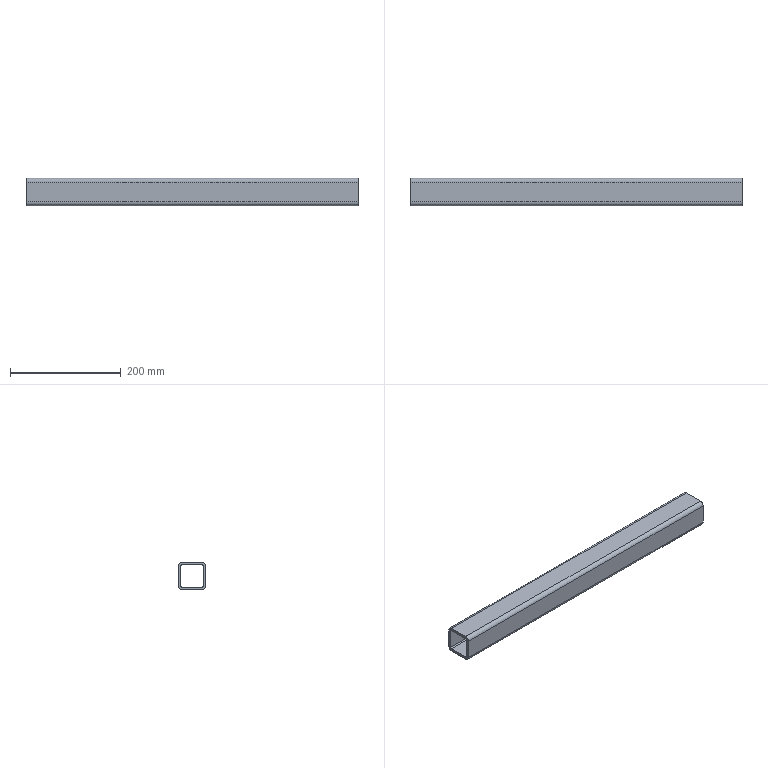Part | NX | 1 solid | 18 faces | box 600 x 50 x 50 mm | volume 516823 mm3 | plane 10 | cylinder 8 | commonest cylinder face diameters 4 x4 14 x4
STEP:
#1=CARTESIAN_POINT('',(950.,838.,20.));
#2=VERTEX_POINT('',#1);
#3=CARTESIAN_POINT('',(350.,838.,20.));
#4=VERTEX_POINT('',#3);
#5=CARTESIAN_POINT('',(975.,838.,20.));
#6=DIRECTION('',(-1.,0.,0.));
#7=VECTOR('',#6,1000.);
#8=LINE('',#5,#7);
#9=EDGE_CURVE('',#2,#4,#8,.T.);
#10=ORIENTED_EDGE('',*,*,#9,.T.);
#11=CARTESIAN_POINT('',(350.,874.,20.));
#12=VERTEX_POINT('',#11);
#13=CARTESIAN_POINT('',(350.,838.,20.));
#14=DIRECTION('',(0.,1.,0.));
#15=VECTOR('',#14,1000.);
#16=LINE('',#13,#15);
#17=EDGE_CURVE('',#4,#12,#16,.T.);
#18=ORIENTED_EDGE('',*,*,#17,.T.);
#19=CARTESIAN_POINT('',(950.,874.,20.));
#20=VERTEX_POINT('',#19);
#21=CARTESIAN_POINT('',(975.,874.,20.));
#22=DIRECTION('',(-1.,0.,0.));
#23=VECTOR('',#22,1000.);
#24=LINE('',#21,#23);
#25=EDGE_CURVE('',#20,#12,#24,.T.);
#26=ORIENTED_EDGE('',*,*,#25,.F.);
#27=CARTESIAN_POINT('',(950.,838.,20.));
#28=DIRECTION('',(0.,-1.,0.));
#29=VECTOR('',#28,1000.);
#30=LINE('',#27,#29);
#31=EDGE_CURVE('',#20,#2,#30,.T.);
#32=ORIENTED_EDGE('',*,*,#31,.T.);
#33=EDGE_LOOP('',(#10,#18,#26,#32));
#34=FACE_BOUND('',#33,.T.);
#35=CARTESIAN_POINT('',(975.,838.,20.));
#36=DIRECTION('',(0.,0.,-1.));
#37=DIRECTION('',(0.,1.,0.));
#38=AXIS2_PLACEMENT_3D('',#35,#36,#37);
#39=PLANE('',#38);
#40=ADVANCED_FACE('',(#34),#39,.T.);
#41=CARTESIAN_POINT('',(950.,836.,18.));
#42=VERTEX_POINT('',#41);
#43=CARTESIAN_POINT('',(350.,836.,18.));
#44=VERTEX_POINT('',#43);
#45=CARTESIAN_POINT('',(975.,836.,18.));
#46=DIRECTION('',(-1.,0.,0.));
#47=VECTOR('',#46,1000.);
#48=LINE('',#45,#47);
#49=EDGE_CURVE('',#42,#44,#48,.T.);
#50=ORIENTED_EDGE('',*,*,#49,.T.);
#51=CARTESIAN_POINT('',(350.,838.,18.));
#52=DIRECTION('',(-1.,0.,0.));
#53=DIRECTION('',(0.,-1.,0.));
#54=AXIS2_PLACEMENT_3D('',#51,#52,#53);
#55=CIRCLE('',#54,2.);
#56=EDGE_CURVE('',#44,#4,#55,.T.);
#57=ORIENTED_EDGE('',*,*,#56,.T.);
#58=ORIENTED_EDGE('',*,*,#9,.F.);
#59=CARTESIAN_POINT('',(950.,838.,18.));
#60=DIRECTION('',(1.,0.,0.));
#61=DIRECTION('',(0.,1.,0.));
#62=AXIS2_PLACEMENT_3D('',#59,#60,#61);
#63=CIRCLE('',#62,2.);
#64=EDGE_CURVE('',#2,#42,#63,.T.);
#65=ORIENTED_EDGE('',*,*,#64,.T.);
#66=EDGE_LOOP('',(#50,#57,#58,#65));
#67=FACE_BOUND('',#66,.T.);
#68=CARTESIAN_POINT('',(975.,838.,18.));
#69=DIRECTION('',(-1.,0.,0.));
#70=DIRECTION('',(0.,0.,1.));
#71=AXIS2_PLACEMENT_3D('',#68,#69,#70);
#72=CYLINDRICAL_SURFACE('',#71,2.);
#73=ADVANCED_FACE('',(#67),#72,.F.);
#74=CARTESIAN_POINT('',(950.,836.,-18.));
#75=VERTEX_POINT('',#74);
#76=CARTESIAN_POINT('',(350.,836.,-18.));
#77=VERTEX_POINT('',#76);
#78=CARTESIAN_POINT('',(975.,836.,-18.));
#79=DIRECTION('',(-1.,0.,0.));
#80=VECTOR('',#79,1000.);
#81=LINE('',#78,#80);
#82=EDGE_CURVE('',#75,#77,#81,.T.);
#83=ORIENTED_EDGE('',*,*,#82,.T.);
#84=CARTESIAN_POINT('',(350.,836.,18.));
#85=DIRECTION('',(0.,0.,1.));
#86=VECTOR('',#85,1000.);
#87=LINE('',#84,#86);
#88=EDGE_CURVE('',#77,#44,#87,.T.);
#89=ORIENTED_EDGE('',*,*,#88,.T.);
#90=ORIENTED_EDGE('',*,*,#49,.F.);
#91=CARTESIAN_POINT('',(950.,836.,18.));
#92=DIRECTION('',(0.,0.,-1.));
#93=VECTOR('',#92,1000.);
#94=LINE('',#91,#93);
#95=EDGE_CURVE('',#42,#75,#94,.T.);
#96=ORIENTED_EDGE('',*,*,#95,.T.);
#97=EDGE_LOOP('',(#83,#89,#90,#96));
#98=FACE_BOUND('',#97,.T.);
#99=CARTESIAN_POINT('',(975.,836.,18.));
#100=DIRECTION('',(0.,1.,0.));
#101=DIRECTION('',(0.,0.,1.));
#102=AXIS2_PLACEMENT_3D('',#99,#100,#101);
#103=PLANE('',#102);
#104=ADVANCED_FACE('',(#98),#103,.T.);
#105=CARTESIAN_POINT('',(950.,838.,-20.));
#106=VERTEX_POINT('',#105);
#107=CARTESIAN_POINT('',(350.,838.,-20.));
#108=VERTEX_POINT('',#107);
#109=CARTESIAN_POINT('',(975.,838.,-20.));
#110=DIRECTION('',(-1.,0.,0.));
#111=VECTOR('',#110,1000.);
#112=LINE('',#109,#111);
#113=EDGE_CURVE('',#106,#108,#112,.T.);
#114=ORIENTED_EDGE('',*,*,#113,.T.);
#115=CARTESIAN_POINT('',(350.,838.,-18.));
#116=DIRECTION('',(-1.,0.,0.));
#117=DIRECTION('',(0.,-1.,0.));
#118=AXIS2_PLACEMENT_3D('',#115,#116,#117);
#119=CIRCLE('',#118,2.);
#120=EDGE_CURVE('',#108,#77,#119,.T.);
#121=ORIENTED_EDGE('',*,*,#120,.T.);
#122=ORIENTED_EDGE('',*,*,#82,.F.);
#123=CARTESIAN_POINT('',(950.,838.,-18.));
#124=DIRECTION('',(1.,0.,0.));
#125=DIRECTION('',(0.,1.,0.));
#126=AXIS2_PLACEMENT_3D('',#123,#124,#125);
#127=CIRCLE('',#126,2.);
#128=EDGE_CURVE('',#75,#106,#127,.T.);
#129=ORIENTED_EDGE('',*,*,#128,.T.);
#130=EDGE_LOOP('',(#114,#121,#122,#129));
#131=FACE_BOUND('',#130,.T.);
#132=CARTESIAN_POINT('',(975.,838.,-18.));
#133=DIRECTION('',(-1.,0.,0.));
#134=DIRECTION('',(0.,0.,1.));
#135=AXIS2_PLACEMENT_3D('',#132,#133,#134);
#136=CYLINDRICAL_SURFACE('',#135,2.);
#137=ADVANCED_FACE('',(#131),#136,.F.);
#138=CARTESIAN_POINT('',(950.,874.,-20.));
#139=VERTEX_POINT('',#138);
#140=CARTESIAN_POINT('',(350.,874.,-20.));
#141=VERTEX_POINT('',#140);
#142=CARTESIAN_POINT('',(975.,874.,-20.));
#143=DIRECTION('',(-1.,0.,0.));
#144=VECTOR('',#143,1000.);
#145=LINE('',#142,#144);
#146=EDGE_CURVE('',#139,#141,#145,.T.);
#147=ORIENTED_EDGE('',*,*,#146,.T.);
#148=CARTESIAN_POINT('',(350.,874.,-20.));
#149=DIRECTION('',(0.,-1.,0.));
#150=VECTOR('',#149,1000.);
#151=LINE('',#148,#150);
#152=EDGE_CURVE('',#141,#108,#151,.T.);
#153=ORIENTED_EDGE('',*,*,#152,.T.);
#154=ORIENTED_EDGE('',*,*,#113,.F.);
#155=CARTESIAN_POINT('',(950.,874.,-20.));
#156=DIRECTION('',(0.,1.,0.));
#157=VECTOR('',#156,1000.);
#158=LINE('',#155,#157);
#159=EDGE_CURVE('',#106,#139,#158,.T.);
#160=ORIENTED_EDGE('',*,*,#159,.T.);
#161=EDGE_LOOP('',(#147,#153,#154,#160));
#162=FACE_BOUND('',#161,.T.);
#163=CARTESIAN_POINT('',(975.,874.,-20.));
#164=DIRECTION('',(0.,0.,1.));
#165=DIRECTION('',(0.,-1.,0.));
#166=AXIS2_PLACEMENT_3D('',#163,#164,#165);
#167=PLANE('',#166);
#168=ADVANCED_FACE('',(#162),#167,.T.);
#169=CARTESIAN_POINT('',(950.,876.,-18.));
#170=VERTEX_POINT('',#169);
#171=CARTESIAN_POINT('',(350.,876.,-18.));
#172=VERTEX_POINT('',#171);
#173=CARTESIAN_POINT('',(975.,876.,-18.));
#174=DIRECTION('',(-1.,0.,0.));
#175=VECTOR('',#174,1000.);
#176=LINE('',#173,#175);
#177=EDGE_CURVE('',#170,#172,#176,.T.);
#178=ORIENTED_EDGE('',*,*,#177,.T.);
#179=CARTESIAN_POINT('',(350.,874.,-18.));
#180=DIRECTION('',(-1.,0.,0.));
#181=DIRECTION('',(0.,-1.,0.));
#182=AXIS2_PLACEMENT_3D('',#179,#180,#181);
#183=CIRCLE('',#182,2.);
#184=EDGE_CURVE('',#172,#141,#183,.T.);
#185=ORIENTED_EDGE('',*,*,#184,.T.);
#186=ORIENTED_EDGE('',*,*,#146,.F.);
#187=CARTESIAN_POINT('',(950.,874.,-18.));
#188=DIRECTION('',(1.,0.,0.));
#189=DIRECTION('',(0.,1.,0.));
#190=AXIS2_PLACEMENT_3D('',#187,#188,#189);
#191=CIRCLE('',#190,2.);
#192=EDGE_CURVE('',#139,#170,#191,.T.);
#193=ORIENTED_EDGE('',*,*,#192,.T.);
#194=EDGE_LOOP('',(#178,#185,#186,#193));
#195=FACE_BOUND('',#194,.T.);
#196=CARTESIAN_POINT('',(975.,874.,-18.));
#197=DIRECTION('',(-1.,0.,0.));
#198=DIRECTION('',(0.,0.,1.));
#199=AXIS2_PLACEMENT_3D('',#196,#197,#198);
#200=CYLINDRICAL_SURFACE('',#199,2.);
#201=ADVANCED_FACE('',(#195),#200,.F.);
#202=CARTESIAN_POINT('',(950.,876.,18.));
#203=VERTEX_POINT('',#202);
#204=CARTESIAN_POINT('',(350.,876.,18.));
#205=VERTEX_POINT('',#204);
#206=CARTESIAN_POINT('',(975.,876.,18.));
#207=DIRECTION('',(-1.,0.,0.));
#208=VECTOR('',#207,1000.);
#209=LINE('',#206,#208);
#210=EDGE_CURVE('',#203,#205,#209,.T.);
#211=ORIENTED_EDGE('',*,*,#210,.T.);
#212=CARTESIAN_POINT('',(350.,876.,-18.));
#213=DIRECTION('',(0.,0.,-1.));
#214=VECTOR('',#213,1000.);
#215=LINE('',#212,#214);
#216=EDGE_CURVE('',#205,#172,#215,.T.);
#217=ORIENTED_EDGE('',*,*,#216,.T.);
#218=ORIENTED_EDGE('',*,*,#177,.F.);
#219=CARTESIAN_POINT('',(950.,876.,-18.));
#220=DIRECTION('',(0.,0.,1.));
#221=VECTOR('',#220,1000.);
#222=LINE('',#219,#221);
#223=EDGE_CURVE('',#170,#203,#222,.T.);
#224=ORIENTED_EDGE('',*,*,#223,.T.);
#225=EDGE_LOOP('',(#211,#217,#218,#224));
#226=FACE_BOUND('',#225,.T.);
#227=CARTESIAN_POINT('',(975.,876.,-18.));
#228=DIRECTION('',(0.,-1.,0.));
#229=DIRECTION('',(0.,0.,-1.));
#230=AXIS2_PLACEMENT_3D('',#227,#228,#229);
#231=PLANE('',#230);
#232=ADVANCED_FACE('',(#226),#231,.T.);
#233=ORIENTED_EDGE('',*,*,#25,.T.);
#234=CARTESIAN_POINT('',(350.,874.,18.));
#235=DIRECTION('',(-1.,0.,0.));
#236=DIRECTION('',(0.,-1.,0.));
#237=AXIS2_PLACEMENT_3D('',#234,#235,#236);
#238=CIRCLE('',#237,2.);
#239=EDGE_CURVE('',#12,#205,#238,.T.);
#240=ORIENTED_EDGE('',*,*,#239,.T.);
#241=ORIENTED_EDGE('',*,*,#210,.F.);
#242=CARTESIAN_POINT('',(950.,874.,18.));
#243=DIRECTION('',(1.,0.,0.));
#244=DIRECTION('',(0.,1.,0.));
#245=AXIS2_PLACEMENT_3D('',#242,#243,#244);
#246=CIRCLE('',#245,2.);
#247=EDGE_CURVE('',#203,#20,#246,.T.);
#248=ORIENTED_EDGE('',*,*,#247,.T.);
#249=EDGE_LOOP('',(#233,#240,#241,#248));
#250=FACE_BOUND('',#249,.T.);
#251=CARTESIAN_POINT('',(975.,874.,18.));
#252=DIRECTION('',(-1.,0.,0.));
#253=DIRECTION('',(0.,0.,1.));
#254=AXIS2_PLACEMENT_3D('',#251,#252,#253);
#255=CYLINDRICAL_SURFACE('',#254,2.);
#256=ADVANCED_FACE('',(#250),#255,.F.);
#257=CARTESIAN_POINT('',(350.,874.,-25.));
#258=VERTEX_POINT('',#257);
#259=CARTESIAN_POINT('',(350.,838.,-25.));
#260=VERTEX_POINT('',#259);
#261=CARTESIAN_POINT('',(350.,874.,-25.));
#262=DIRECTION('',(0.,-1.,0.));
#263=VECTOR('',#262,1000.);
#264=LINE('',#261,#263);
#265=EDGE_CURVE('',#258,#260,#264,.T.);
#266=ORIENTED_EDGE('',*,*,#265,.F.);
#267=CARTESIAN_POINT('',(950.,874.,-25.));
#268=VERTEX_POINT('',#267);
#269=CARTESIAN_POINT('',(975.,874.,-25.));
#270=DIRECTION('',(-1.,0.,0.));
#271=VECTOR('',#270,1000.);
#272=LINE('',#269,#271);
#273=EDGE_CURVE('',#268,#258,#272,.T.);
#274=ORIENTED_EDGE('',*,*,#273,.F.);
#275=CARTESIAN_POINT('',(950.,838.,-25.));
#276=VERTEX_POINT('',#275);
#277=CARTESIAN_POINT('',(950.,874.,-25.));
#278=DIRECTION('',(0.,1.,0.));
#279=VECTOR('',#278,1000.);
#280=LINE('',#277,#279);
#281=EDGE_CURVE('',#276,#268,#280,.T.);
#282=ORIENTED_EDGE('',*,*,#281,.F.);
#283=CARTESIAN_POINT('',(975.,838.,-25.));
#284=DIRECTION('',(-1.,0.,0.));
#285=VECTOR('',#284,1000.);
#286=LINE('',#283,#285);
#287=EDGE_CURVE('',#276,#260,#286,.T.);
#288=ORIENTED_EDGE('',*,*,#287,.T.);
#289=EDGE_LOOP('',(#266,#274,#282,#288));
#290=FACE_BOUND('',#289,.T.);
#291=CARTESIAN_POINT('',(975.,874.,-25.));
#292=DIRECTION('',(0.,0.,1.));
#293=DIRECTION('',(0.,-1.,0.));
#294=AXIS2_PLACEMENT_3D('',#291,#292,#293);
#295=PLANE('',#294);
#296=ADVANCED_FACE('',(#290),#295,.F.);
#297=CARTESIAN_POINT('',(350.,831.,-18.));
#298=VERTEX_POINT('',#297);
#299=CARTESIAN_POINT('',(350.,838.,-18.));
#300=DIRECTION('',(-1.,0.,0.));
#301=DIRECTION('',(0.,-1.,0.));
#302=AXIS2_PLACEMENT_3D('',#299,#300,#301);
#303=CIRCLE('',#302,7.);
#304=EDGE_CURVE('',#260,#298,#303,.T.);
#305=ORIENTED_EDGE('',*,*,#304,.F.);
#306=ORIENTED_EDGE('',*,*,#287,.F.);
#307=CARTESIAN_POINT('',(950.,831.,-18.));
#308=VERTEX_POINT('',#307);
#309=CARTESIAN_POINT('',(950.,838.,-18.));
#310=DIRECTION('',(1.,0.,0.));
#311=DIRECTION('',(0.,1.,0.));
#312=AXIS2_PLACEMENT_3D('',#309,#310,#311);
#313=CIRCLE('',#312,7.);
#314=EDGE_CURVE('',#308,#276,#313,.T.);
#315=ORIENTED_EDGE('',*,*,#314,.F.);
#316=CARTESIAN_POINT('',(975.,831.,-18.));
#317=DIRECTION('',(-1.,0.,0.));
#318=VECTOR('',#317,1000.);
#319=LINE('',#316,#318);
#320=EDGE_CURVE('',#308,#298,#319,.T.);
#321=ORIENTED_EDGE('',*,*,#320,.T.);
#322=EDGE_LOOP('',(#305,#306,#315,#321));
#323=FACE_BOUND('',#322,.T.);
#324=CARTESIAN_POINT('',(975.,838.,-18.));
#325=DIRECTION('',(-1.,0.,0.));
#326=DIRECTION('',(0.,0.,1.));
#327=AXIS2_PLACEMENT_3D('',#324,#325,#326);
#328=CYLINDRICAL_SURFACE('',#327,7.);
#329=ADVANCED_FACE('',(#323),#328,.T.);
#330=CARTESIAN_POINT('',(350.,831.,18.));
#331=VERTEX_POINT('',#330);
#332=CARTESIAN_POINT('',(350.,831.,575.));
#333=DIRECTION('',(0.,0.,-1.));
#334=VECTOR('',#333,1000.);
#335=LINE('',#332,#334);
#336=EDGE_CURVE('',#331,#298,#335,.T.);
#337=ORIENTED_EDGE('',*,*,#336,.T.);
#338=ORIENTED_EDGE('',*,*,#320,.F.);
#339=CARTESIAN_POINT('',(950.,831.,18.));
#340=VERTEX_POINT('',#339);
#341=CARTESIAN_POINT('',(950.,831.,575.));
#342=DIRECTION('',(0.,0.,-1.));
#343=VECTOR('',#342,1000.);
#344=LINE('',#341,#343);
#345=EDGE_CURVE('',#340,#308,#344,.T.);
#346=ORIENTED_EDGE('',*,*,#345,.F.);
#347=CARTESIAN_POINT('',(975.,831.,18.));
#348=DIRECTION('',(-1.,0.,0.));
#349=VECTOR('',#348,1000.);
#350=LINE('',#347,#349);
#351=EDGE_CURVE('',#340,#331,#350,.T.);
#352=ORIENTED_EDGE('',*,*,#351,.T.);
#353=EDGE_LOOP('',(#337,#338,#346,#352));
#354=FACE_BOUND('',#353,.T.);
#355=CARTESIAN_POINT('',(975.,831.,18.));
#356=DIRECTION('',(0.,1.,0.));
#357=DIRECTION('',(0.,0.,1.));
#358=AXIS2_PLACEMENT_3D('',#355,#356,#357);
#359=PLANE('',#358);
#360=ADVANCED_FACE('',(#354),#359,.F.);
#361=CARTESIAN_POINT('',(350.,838.,25.));
#362=VERTEX_POINT('',#361);
#363=CARTESIAN_POINT('',(350.,838.,18.));
#364=DIRECTION('',(-1.,0.,0.));
#365=DIRECTION('',(0.,-1.,0.));
#366=AXIS2_PLACEMENT_3D('',#363,#364,#365);
#367=CIRCLE('',#366,7.);
#368=EDGE_CURVE('',#331,#362,#367,.T.);
#369=ORIENTED_EDGE('',*,*,#368,.F.);
#370=ORIENTED_EDGE('',*,*,#351,.F.);
#371=CARTESIAN_POINT('',(950.,838.,25.));
#372=VERTEX_POINT('',#371);
#373=CARTESIAN_POINT('',(950.,838.,18.));
#374=DIRECTION('',(1.,0.,0.));
#375=DIRECTION('',(0.,1.,0.));
#376=AXIS2_PLACEMENT_3D('',#373,#374,#375);
#377=CIRCLE('',#376,7.);
#378=EDGE_CURVE('',#372,#340,#377,.T.);
#379=ORIENTED_EDGE('',*,*,#378,.F.);
#380=CARTESIAN_POINT('',(975.,838.,25.));
#381=DIRECTION('',(-1.,0.,0.));
#382=VECTOR('',#381,1000.);
#383=LINE('',#380,#382);
#384=EDGE_CURVE('',#372,#362,#383,.T.);
#385=ORIENTED_EDGE('',*,*,#384,.T.);
#386=EDGE_LOOP('',(#369,#370,#379,#385));
#387=FACE_BOUND('',#386,.T.);
#388=CARTESIAN_POINT('',(975.,838.,18.));
#389=DIRECTION('',(-1.,0.,0.));
#390=DIRECTION('',(0.,0.,1.));
#391=AXIS2_PLACEMENT_3D('',#388,#389,#390);
#392=CYLINDRICAL_SURFACE('',#391,7.);
#393=ADVANCED_FACE('',(#387),#392,.T.);
#394=CARTESIAN_POINT('',(350.,874.,25.));
#395=VERTEX_POINT('',#394);
#396=CARTESIAN_POINT('',(350.,838.,25.));
#397=DIRECTION('',(0.,1.,0.));
#398=VECTOR('',#397,1000.);
#399=LINE('',#396,#398);
#400=EDGE_CURVE('',#362,#395,#399,.T.);
#401=ORIENTED_EDGE('',*,*,#400,.F.);
#402=ORIENTED_EDGE('',*,*,#384,.F.);
#403=CARTESIAN_POINT('',(950.,874.,25.));
#404=VERTEX_POINT('',#403);
#405=CARTESIAN_POINT('',(950.,838.,25.));
#406=DIRECTION('',(0.,-1.,0.));
#407=VECTOR('',#406,1000.);
#408=LINE('',#405,#407);
#409=EDGE_CURVE('',#404,#372,#408,.T.);
#410=ORIENTED_EDGE('',*,*,#409,.F.);
#411=CARTESIAN_POINT('',(975.,874.,25.));
#412=DIRECTION('',(-1.,0.,0.));
#413=VECTOR('',#412,1000.);
#414=LINE('',#411,#413);
#415=EDGE_CURVE('',#404,#395,#414,.T.);
#416=ORIENTED_EDGE('',*,*,#415,.T.);
#417=EDGE_LOOP('',(#401,#402,#410,#416));
#418=FACE_BOUND('',#417,.T.);
#419=CARTESIAN_POINT('',(975.,838.,25.));
#420=DIRECTION('',(0.,0.,-1.));
#421=DIRECTION('',(0.,1.,0.));
#422=AXIS2_PLACEMENT_3D('',#419,#420,#421);
#423=PLANE('',#422);
#424=ADVANCED_FACE('',(#418),#423,.F.);
#425=CARTESIAN_POINT('',(350.,881.,18.));
#426=VERTEX_POINT('',#425);
#427=CARTESIAN_POINT('',(350.,874.,18.));
#428=DIRECTION('',(-1.,0.,0.));
#429=DIRECTION('',(0.,-1.,0.));
#430=AXIS2_PLACEMENT_3D('',#427,#428,#429);
#431=CIRCLE('',#430,7.);
#432=EDGE_CURVE('',#395,#426,#431,.T.);
#433=ORIENTED_EDGE('',*,*,#432,.F.);
#434=ORIENTED_EDGE('',*,*,#415,.F.);
#435=CARTESIAN_POINT('',(950.,881.,18.));
#436=VERTEX_POINT('',#435);
#437=CARTESIAN_POINT('',(950.,874.,18.));
#438=DIRECTION('',(1.,0.,0.));
#439=DIRECTION('',(0.,1.,0.));
#440=AXIS2_PLACEMENT_3D('',#437,#438,#439);
#441=CIRCLE('',#440,7.);
#442=EDGE_CURVE('',#436,#404,#441,.T.);
#443=ORIENTED_EDGE('',*,*,#442,.F.);
#444=CARTESIAN_POINT('',(975.,881.,18.));
#445=DIRECTION('',(-1.,0.,0.));
#446=VECTOR('',#445,1000.);
#447=LINE('',#444,#446);
#448=EDGE_CURVE('',#436,#426,#447,.T.);
#449=ORIENTED_EDGE('',*,*,#448,.T.);
#450=EDGE_LOOP('',(#433,#434,#443,#449));
#451=FACE_BOUND('',#450,.T.);
#452=CARTESIAN_POINT('',(975.,874.,18.));
#453=DIRECTION('',(-1.,0.,0.));
#454=DIRECTION('',(0.,0.,1.));
#455=AXIS2_PLACEMENT_3D('',#452,#453,#454);
#456=CYLINDRICAL_SURFACE('',#455,7.);
#457=ADVANCED_FACE('',(#451),#456,.T.);
#458=CARTESIAN_POINT('',(350.,881.,-18.));
#459=VERTEX_POINT('',#458);
#460=CARTESIAN_POINT('',(350.,881.,575.));
#461=DIRECTION('',(0.,0.,-1.));
#462=VECTOR('',#461,1000.);
#463=LINE('',#460,#462);
#464=EDGE_CURVE('',#426,#459,#463,.T.);
#465=ORIENTED_EDGE('',*,*,#464,.F.);
#466=ORIENTED_EDGE('',*,*,#448,.F.);
#467=CARTESIAN_POINT('',(950.,881.,-18.));
#468=VERTEX_POINT('',#467);
#469=CARTESIAN_POINT('',(950.,881.,575.));
#470=DIRECTION('',(0.,0.,-1.));
#471=VECTOR('',#470,1000.);
#472=LINE('',#469,#471);
#473=EDGE_CURVE('',#436,#468,#472,.T.);
#474=ORIENTED_EDGE('',*,*,#473,.T.);
#475=CARTESIAN_POINT('',(975.,881.,-18.));
#476=DIRECTION('',(-1.,0.,0.));
#477=VECTOR('',#476,1000.);
#478=LINE('',#475,#477);
#479=EDGE_CURVE('',#468,#459,#478,.T.);
#480=ORIENTED_EDGE('',*,*,#479,.T.);
#481=EDGE_LOOP('',(#465,#466,#474,#480));
#482=FACE_BOUND('',#481,.T.);
#483=CARTESIAN_POINT('',(975.,881.,-18.));
#484=DIRECTION('',(0.,-1.,0.));
#485=DIRECTION('',(0.,0.,-1.));
#486=AXIS2_PLACEMENT_3D('',#483,#484,#485);
#487=PLANE('',#486);
#488=ADVANCED_FACE('',(#482),#487,.F.);
#489=CARTESIAN_POINT('',(350.,874.,-18.));
#490=DIRECTION('',(-1.,0.,0.));
#491=DIRECTION('',(0.,-1.,0.));
#492=AXIS2_PLACEMENT_3D('',#489,#490,#491);
#493=CIRCLE('',#492,7.);
#494=EDGE_CURVE('',#459,#258,#493,.T.);
#495=ORIENTED_EDGE('',*,*,#494,.F.);
#496=ORIENTED_EDGE('',*,*,#479,.F.);
#497=CARTESIAN_POINT('',(950.,874.,-18.));
#498=DIRECTION('',(1.,0.,0.));
#499=DIRECTION('',(0.,1.,0.));
#500=AXIS2_PLACEMENT_3D('',#497,#498,#499);
#501=CIRCLE('',#500,7.);
#502=EDGE_CURVE('',#268,#468,#501,.T.);
#503=ORIENTED_EDGE('',*,*,#502,.F.);
#504=ORIENTED_EDGE('',*,*,#273,.T.);
#505=EDGE_LOOP('',(#495,#496,#503,#504));
#506=FACE_BOUND('',#505,.T.);
#507=CARTESIAN_POINT('',(975.,874.,-18.));
#508=DIRECTION('',(-1.,0.,0.));
#509=DIRECTION('',(0.,0.,1.));
#510=AXIS2_PLACEMENT_3D('',#507,#508,#509);
#511=CYLINDRICAL_SURFACE('',#510,7.);
#512=ADVANCED_FACE('',(#506),#511,.T.);
#513=ORIENTED_EDGE('',*,*,#223,.F.);
#514=ORIENTED_EDGE('',*,*,#192,.F.);
#515=ORIENTED_EDGE('',*,*,#159,.F.);
#516=ORIENTED_EDGE('',*,*,#128,.F.);
#517=ORIENTED_EDGE('',*,*,#95,.F.);
#518=ORIENTED_EDGE('',*,*,#64,.F.);
#519=ORIENTED_EDGE('',*,*,#31,.F.);
#520=ORIENTED_EDGE('',*,*,#247,.F.);
#521=EDGE_LOOP('',(#513,#514,#515,#516,#517,#518,#519,#520));
#522=FACE_BOUND('',#521,.T.);
#523=ORIENTED_EDGE('',*,*,#442,.T.);
#524=ORIENTED_EDGE('',*,*,#409,.T.);
#525=ORIENTED_EDGE('',*,*,#378,.T.);
#526=ORIENTED_EDGE('',*,*,#345,.T.);
#527=ORIENTED_EDGE('',*,*,#314,.T.);
#528=ORIENTED_EDGE('',*,*,#281,.T.);
#529=ORIENTED_EDGE('',*,*,#502,.T.);
#530=ORIENTED_EDGE('',*,*,#473,.F.);
#531=EDGE_LOOP('',(#523,#524,#525,#526,#527,#528,#529,#530));
#532=FACE_BOUND('',#531,.T.);
#533=CARTESIAN_POINT('',(950.,838.,575.));
#534=DIRECTION('',(1.,0.,0.));
#535=DIRECTION('',(0.,1.,0.));
#536=AXIS2_PLACEMENT_3D('',#533,#534,#535);
#537=PLANE('',#536);
#538=ADVANCED_FACE('',(#522,#532),#537,.T.);
#539=ORIENTED_EDGE('',*,*,#56,.F.);
#540=ORIENTED_EDGE('',*,*,#88,.F.);
#541=ORIENTED_EDGE('',*,*,#120,.F.);
#542=ORIENTED_EDGE('',*,*,#152,.F.);
#543=ORIENTED_EDGE('',*,*,#184,.F.);
#544=ORIENTED_EDGE('',*,*,#216,.F.);
#545=ORIENTED_EDGE('',*,*,#239,.F.);
#546=ORIENTED_EDGE('',*,*,#17,.F.);
#547=EDGE_LOOP('',(#539,#540,#541,#542,#543,#544,#545,#546));
#548=FACE_BOUND('',#547,.T.);
#549=ORIENTED_EDGE('',*,*,#368,.T.);
#550=ORIENTED_EDGE('',*,*,#400,.T.);
#551=ORIENTED_EDGE('',*,*,#432,.T.);
#552=ORIENTED_EDGE('',*,*,#464,.T.);
#553=ORIENTED_EDGE('',*,*,#494,.T.);
#554=ORIENTED_EDGE('',*,*,#265,.T.);
#555=ORIENTED_EDGE('',*,*,#304,.T.);
#556=ORIENTED_EDGE('',*,*,#336,.F.);
#557=EDGE_LOOP('',(#549,#550,#551,#552,#553,#554,#555,#556));
#558=FACE_BOUND('',#557,.T.);
#559=CARTESIAN_POINT('',(350.,874.,575.));
#560=DIRECTION('',(-1.,0.,0.));
#561=DIRECTION('',(0.,-1.,0.));
#562=AXIS2_PLACEMENT_3D('',#559,#560,#561);
#563=PLANE('',#562);
#564=ADVANCED_FACE('',(#548,#558),#563,.T.);
#565=CLOSED_SHELL('',(#40,#73,#104,#137,#168,#201,#232,#256,#296,#329,#360,#393,#424,#457,#488,#512,#538,#564));
#566=MANIFOLD_SOLID_BREP('',#565);
#567=(LENGTH_UNIT()NAMED_UNIT(*)SI_UNIT(.MILLI.,.METRE.));
#568=UNCERTAINTY_MEASURE_WITH_UNIT(LENGTH_MEASURE(0.00001),#567,'','');
#569=(NAMED_UNIT(*)PLANE_ANGLE_UNIT()SI_UNIT($,.RADIAN.));
#570=(NAMED_UNIT(*)SI_UNIT($,.STERADIAN.)SOLID_ANGLE_UNIT());
#571=(GEOMETRIC_REPRESENTATION_CONTEXT(3)GLOBAL_UNCERTAINTY_ASSIGNED_CONTEXT((#568))GLOBAL_UNIT_ASSIGNED_CONTEXT((#567,#569,#570))REPRESENTATION_CONTEXT('',''));
#572=ADVANCED_BREP_SHAPE_REPRESENTATION('',(#566),#571);